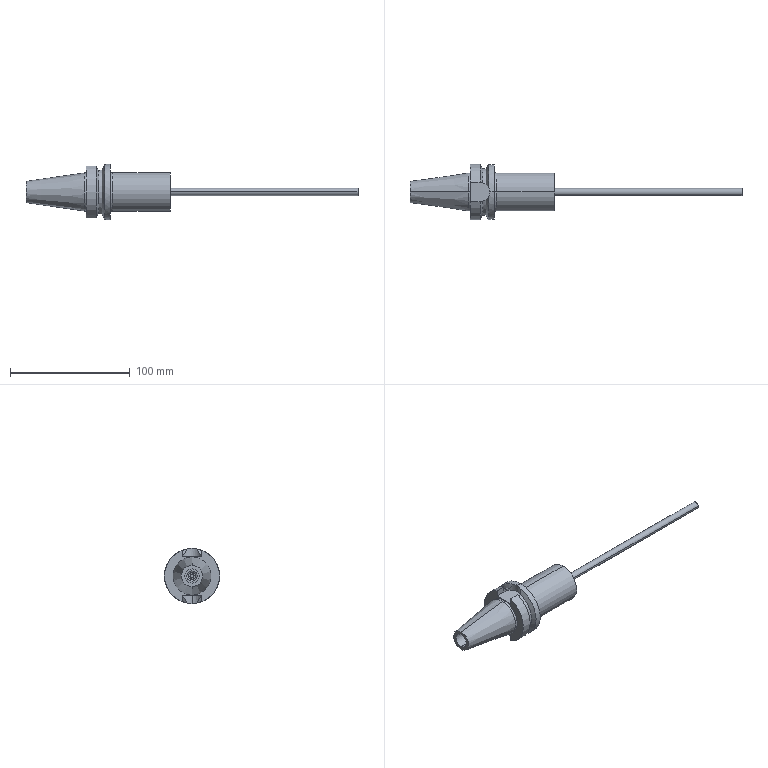Part | SolidWorks | features BaseBody 10 | 9 solids | 104 faces | box 277 x 46 x 46 mm | volume 91499 mm3 | plane 41 | cylinder 39 | cone 16 | torus 8 | commonest cylinder face diameters 3 x6 21 x6 6 x4 46 x4 16.1 x3 8.5 x2